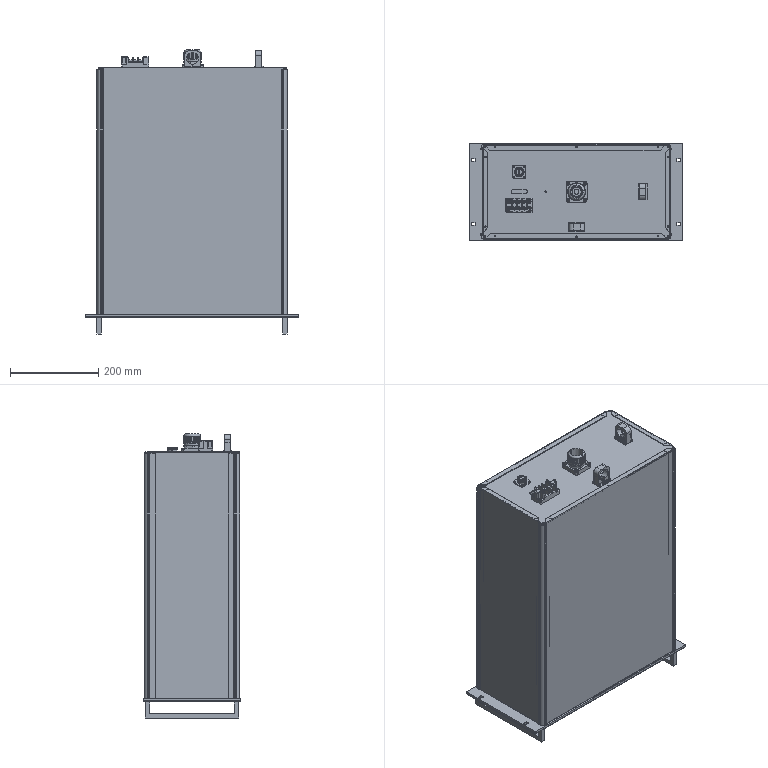Part | SolidWorks | features BaseBody 11 | 11 solids | 2007 faces | box 483 x 221.8 x 643.931 mm | volume 2898841 mm3 | plane 1114 | cylinder 693 | spline 159 | cone 17 | sphere 14 | torus 10 | commonest cylinder face diameters 3 x368 3.3 x70 10 x37 4 x34 3.5 x28 6 x19